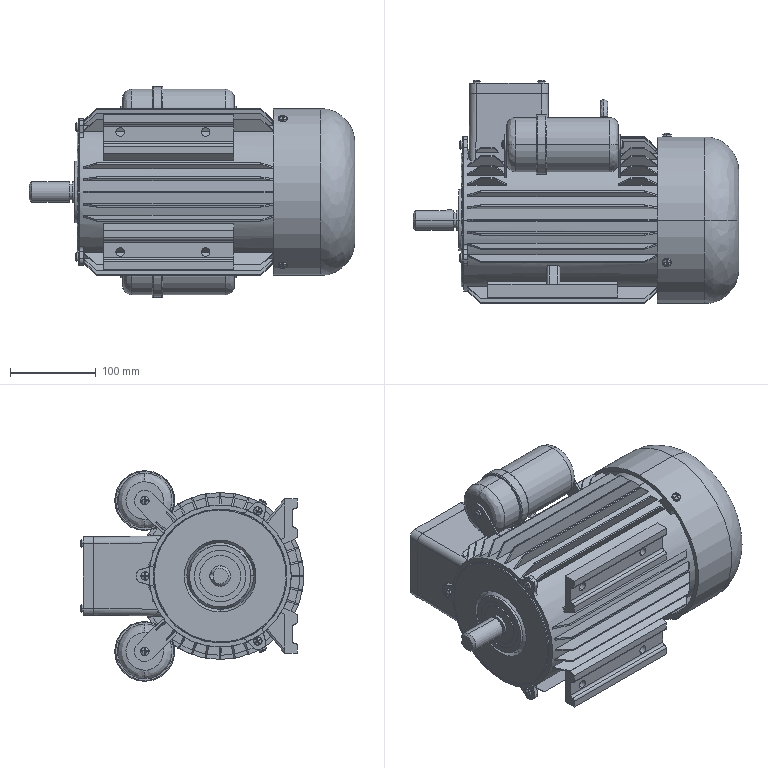Part | SolidWorks | features BaseBody 4 | 4 solids | 739 faces | box 380 x 260.832 x 246 mm | volume 9231400 mm3 | plane 385 | cylinder 181 | cone 87 | spline 86 | commonest cylinder face diameters 10 x56 195 x51 5.625 x12 24 x10 8.444 x8 16 x8